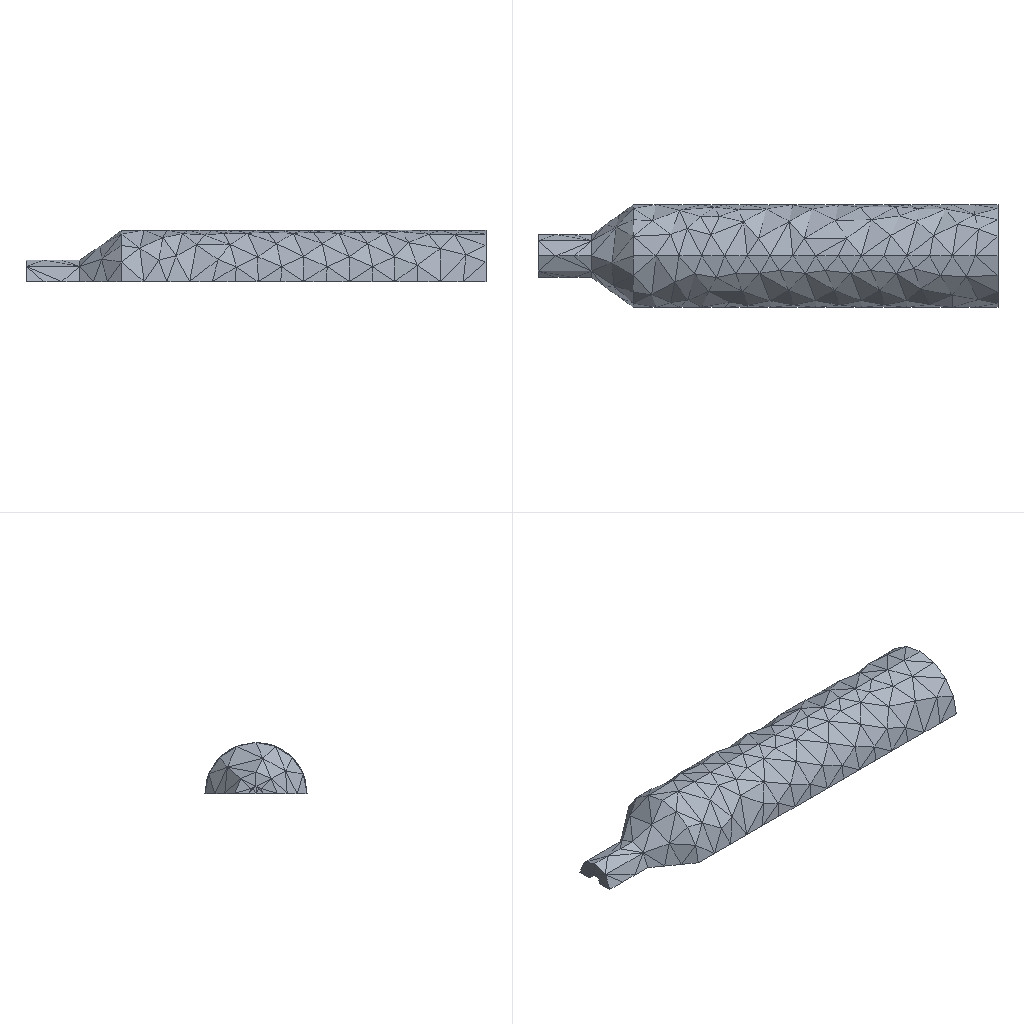Simulation study | ansys workbench
Ansys APDL input file, long lists of numbers shortened:
/batch
/config,noeldb,1     ! force off writing results to database
*get,_wallstrt,active,,time,wall
! ANSYS input file written by Workbench version 2022 R1
! File used for geometry attach:
/title,wbnew--____ (B5)
! ****** Begin Custom Load Command Snippet ******
/COM, ACT Extensions:
/COM,     LSDYNA, 2021.1
/COM,
! ****** End   Custom Load Command Snippet ******
*DIM,_wb_ProjectScratch_dir,string,248
_wb_ProjectScratch_dir(1) = ''
*DIM,_wb_SolverFiles_dir,string,248
_wb_SolverFiles_dir(1) = ''
*DIM,_wb_userfiles_dir,string,248
_wb_userfiles_dir(1) = ''
/com,--- Data in consistent NMM units. See Solving Units in the help system for more information.
/units,MPA
/nopr
/wb,file,start              !  signify a WB generated input file
/prep7
! Turn off shape checking because checks already performed inside WB mesher.
! See help system for more information.
SHPP,OFF,,NOWARN
/nolist
etcon,set             ! allow ANSYS to choose best KEYOP's for 180x elements, resets any applicable keyopt to MAPDL defaults
/com,*********** Nodes for the whole assembly ***********
nblock,3,,1742
(1i9,3e20.9e3)
        1     1.249000000E+03     0.000000000E+00     1.043258926E+02
! (1583 more lines like these left out)
-1
/wb,elem,start            !  set before creation of elements
/com,*********** Elements for Body 1 "__2-FreeParts|__-__2" ***********
et,1,187
eblock,19,solid,,716
(19i9)
        1        1        1        1        0        0        0        0       10        0        1       16      197      253       17      445     1321      447      441
! (1431 more lines like these left out)
-1
/wb,elem,end               !  done creating elements
/com,*********** Send User Defined Coordinate System(s) ***********
csys,0
toffst,273.15,  ! Temperature offset from absolute zero
/com,*********** Set Reference Temperature ***********
tref,22.
/wb,mat,start              !  starting to send materials
/com,*********** Send Materials ***********
Temperature = 'TEMP' ! Temperature
MP,DENS,1,7.85e-09,	! tonne mm^-3
MP,ALPX,1,1.2e-05,	! C^-1
MP,C,1,434000000,	! mm^2 s^-2 C^-1
MP,KXX,1,60.5,	! tonne mm s^-3 C^-1
MP,RSVX,1,0.00017,	! ohm mm
MP,EX,1,200000,	! tonne s^-2 mm^-1
MP,NUXY,1,0.3,
MP,MURX,1,10000,
/wb,mat,end                !  done sending materials
!************************* Model Summary ********************
!__2-FreeParts|__-__2,	结构钢,	matid,	1
!************************* End Model Summary ********************
! get the diagonal of the bounding box. Needed later for other things
*get,_xmin,node,,mnloc,x
*get,_ymin,node,,mnloc,y
*get,_zmin,node,,mnloc,z
*get,_xmax,node,,mxloc,x
*get,_ymax,node,,mxloc,y
*get,_zmax,node,,mxloc,z
_ASMDIAG=(_xmax-_xmin)*(_xmax-_xmin)+(_ymax-_ymin)*(_ymax-_ymin)+(_zmax-_zmin)*(_zmax-_zmin)
_ASMDIAG=SQRT(_ASMDIAG)
/wb,contact,start          !  starting to send contact
/wb,contact,end            !  done creating contacts
/golist
/wb,load,start             !  starting to send loads
/com,*********** Fixed Supports ***********
CMBLOCK,_FIXEDSU,NODE,       36
(8i10)
        57        58        59        60        61        97        98        99
       100       101       102       103       104       718       720       722
       724       725       726       727       729       733       734       735
       741       938       939       941       942       943       945       946
       947       950       958       960
cmsel,s,_FIXEDSU
d,all,all
nsel,all
/com,*********** Define Pressure Using Surface Effect Elements "__" ***********
et,2,154
eblock,10,,,204
(15i9)
     1291        2        2        2        0      102      103      203      203      958      961      203      959
! (203 more lines like these left out)
-1
esel,s,type,,2
keyop,2,7,0                ! Use deformed area for application of load
esel,all
/com,*********** Define Pressure Using Surface Effect Elements "__ 2" ***********
et,3,154
eblock,10,,,160
(15i9)
     1495        3        3        3        0        3        1        6        6      292      293        6      311
! (159 more lines like these left out)
-1
esel,s,type,,3
keyop,3,7,0                ! Use deformed area for application of load
esel,all
esel,all
/gst,on,on
fini
*get,_numnode,node,0,count
*get,_numelem,elem,0,count
*get, _MAXELEMNUM, elem, 0, NUM, MAX
*get, _MAXNODENUM, node, 0, NUM, MAX
*get, _MAXELEMTYPE, etyp, 0, NUM, MAX
*get, _MAXREALCONST, real, 0, NUM, MAX
/go
/wb,load,end               !  done creating loads
/com,--- Number of total nodes = %_numnode%
/com,--- Number of contact elements = 364
/com,--- Number of spring elements = 0
/com,--- Number of bearing elements = 0
/com,--- Number of solid elements = 716
/com,--- Number of condensed parts = 0
/com,--- Number of total elements = %_numelem%
*get,_wallbsol,active,,time,wall
/com,****************************************************************************
/com,*************************    SOLUTION       ********************************
/com,****************************************************************************
/solu
antype,0                   ! static analysis
_thickRatio=  0     ! Ratio of thick parts in the model
eqsl,sparse,,,,,1
cntr,print,1               ! print out contact info and also make no initial contact an error
dmpoption,emat,no             ! Don't combine emat file for DANSYS
dmpoption,esav,no             ! Don't combine esav file for DANSYS
nldiag,cont,iter           ! print out contact info each equilibrium iteration
rescontrol,,none                 ! Do not keep any restart files
/com,****************************************************
/com,******************* SOLVE FOR LS 1 OF 1 ****************
esel,s,type,,2
nsle
sf,all,pres,20.
esel,s,type,,3
nsle
sf,all,pres,60.
nsel,all
esel,all
esel,all
/nopr
/gopr
nsub,1,1,1
time,1.
outres,erase
outres,all,none
outres,nsol,all,
outres,rsol,all
outres,eangl,all
outres,etmp,all
outres,veng,all
outres,strs,all,
outres,epel,all,
outres,eppl,all,
outres,cont,all,
! *********** WB SOLVE COMMAND ***********
! check interactive state
*get,ANSINTER_,active,,int
*if,ANSINTER_,ne,0,then
/eof
*endif
solve
/com *************** Write FE CONNECTORS *********
CEWRITE,file,ce,,INTE
/com,****************************************************
/com,*************** FINISHED SOLVE FOR LS 1 *************
*get,_wallasol,active,,time,wall
/nopr
*get,_numnode,node,0,count
*get,_numelem,elem,0,count
*get, _MAXELEMNUM, elem, 0, NUM, MAX
*get, _MAXNODENUM, node, 0, NUM, MAX,,,INTERNAL
*get, _MAXELEMTYPE, etyp, 0, NUM, MAX
*get, _MAXREALCONST, real, 0, NUM, MAX
/gopr
/post1
xmlo,ENCODING,ISO-8859-1
xmlo,parm
/xml,parm,xml
fini
/gopr
*get,_walldone,active,,time,wall
_preptime=(_wallbsol-_wallstrt)*3600
_solvtime=(_wallasol-_wallbsol)*3600
_posttime=(_walldone-_wallasol)*3600
_totaltim=(_walldone-_wallstrt)*3600
*get,_dlbratio,active,0,solu,dlbr
*get,_combtime,active,0,solu,comb
*get,_ssmode,active,0,solu,ssmm
*get,_ndofs,active,0,solu,ndof
*get,_sol_end_time,active,0,set,time
*if,_sol_end_time,eq,1.,then
/fclean				!clean distributed files
*endif
/com,--- Total number of nodes = %_numnode%
/com,--- Total number of elements = %_numelem%
/com,--- Element load balance ratio = %_dlbratio%
/com,--- Time to combine distributed files = %_combtime%
/com,--- Sparse memory mode = %_ssmode%
/com,--- Number of DOF = %_ndofs%
/wb,file,end               ! done with WB generated input